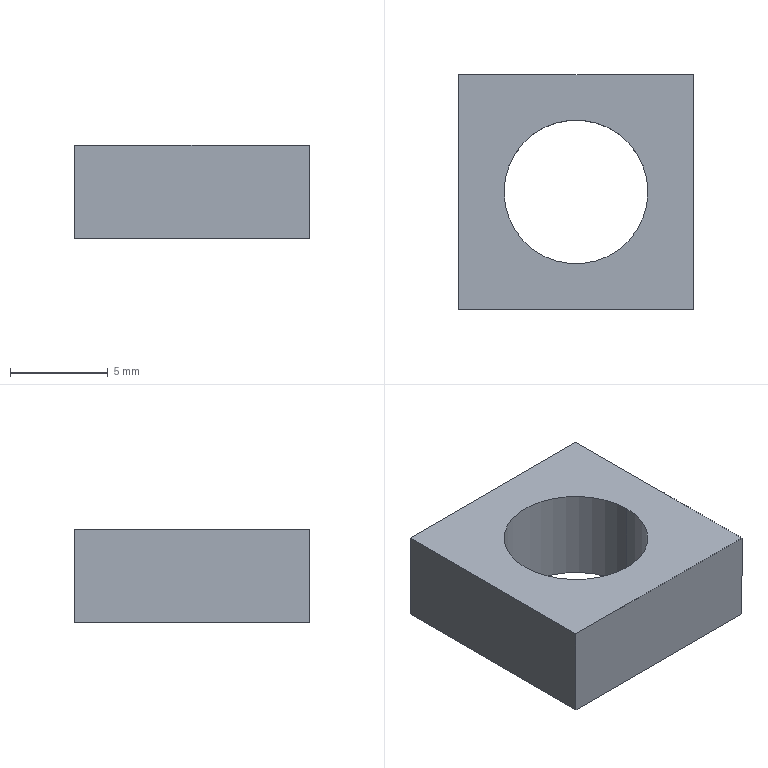Part | SolidWorks | features Extrusion 1 | 1 solid | 8 faces | box 12 x 12 x 4.756 mm | volume 483.113 mm3 | plane 6 | cylinder 2 | commonest cylinder face diameters 7.349 x2
STEP:
#1=CARTESIAN_POINT('',(15.877,1.837,4.756));
#2=VERTEX_POINT('',#1);
#3=CARTESIAN_POINT('',(23.226,1.837,4.756));
#4=VERTEX_POINT('',#3);
#5=CARTESIAN_POINT('',(19.552,1.837,4.756));
#6=DIRECTION('',(0.,0.,1.));
#7=DIRECTION('',(1.,0.,0.));
#8=AXIS2_PLACEMENT_3D('',#5,#6,#7);
#9=CIRCLE('',#8,3.675);
#10=EDGE_CURVE('',#2,#4,#9,.T.);
#11=ORIENTED_EDGE('',*,*,#10,.T.);
#12=CARTESIAN_POINT('',(23.226,1.837,0.));
#13=VERTEX_POINT('',#12);
#14=CARTESIAN_POINT('',(23.226,1.837,21.727));
#15=DIRECTION('',(0.,0.,-1.));
#16=VECTOR('',#15,1000.);
#17=LINE('',#14,#16);
#18=EDGE_CURVE('',#4,#13,#17,.T.);
#19=ORIENTED_EDGE('',*,*,#18,.T.);
#20=CARTESIAN_POINT('',(15.877,1.837,0.));
#21=VERTEX_POINT('',#20);
#22=CARTESIAN_POINT('',(19.552,1.837,0.));
#23=DIRECTION('',(0.,0.,1.));
#24=DIRECTION('',(1.,0.,0.));
#25=AXIS2_PLACEMENT_3D('',#22,#23,#24);
#26=CIRCLE('',#25,3.675);
#27=EDGE_CURVE('',#21,#13,#26,.T.);
#28=ORIENTED_EDGE('',*,*,#27,.F.);
#29=CARTESIAN_POINT('',(15.877,1.837,21.727));
#30=DIRECTION('',(0.,0.,-1.));
#31=VECTOR('',#30,1000.);
#32=LINE('',#29,#31);
#33=EDGE_CURVE('',#2,#21,#32,.T.);
#34=ORIENTED_EDGE('',*,*,#33,.F.);
#35=EDGE_LOOP('',(#11,#19,#28,#34));
#36=FACE_OUTER_BOUND('',#35,.T.);
#37=CARTESIAN_POINT('',(19.552,1.837,21.727));
#38=DIRECTION('',(0.,0.,-1.));
#39=DIRECTION('',(-1.,0.,0.));
#40=AXIS2_PLACEMENT_3D('',#37,#38,#39);
#41=CYLINDRICAL_SURFACE('',#40,3.675);
#42=ADVANCED_FACE('',(#36),#41,.F.);
#43=CARTESIAN_POINT('',(13.552,-4.163,4.756));
#44=VERTEX_POINT('',#43);
#45=CARTESIAN_POINT('',(25.552,-4.163,4.756));
#46=VERTEX_POINT('',#45);
#47=CARTESIAN_POINT('',(13.552,-4.163,4.756));
#48=DIRECTION('',(1.,0.,0.));
#49=VECTOR('',#48,1000.);
#50=LINE('',#47,#49);
#51=EDGE_CURVE('',#44,#46,#50,.T.);
#52=ORIENTED_EDGE('',*,*,#51,.F.);
#53=CARTESIAN_POINT('',(13.552,-4.163,0.));
#54=VERTEX_POINT('',#53);
#55=CARTESIAN_POINT('',(13.552,-4.163,21.727));
#56=DIRECTION('',(0.,0.,-1.));
#57=VECTOR('',#56,1000.);
#58=LINE('',#55,#57);
#59=EDGE_CURVE('',#44,#54,#58,.T.);
#60=ORIENTED_EDGE('',*,*,#59,.T.);
#61=CARTESIAN_POINT('',(25.552,-4.163,0.));
#62=VERTEX_POINT('',#61);
#63=CARTESIAN_POINT('',(13.552,-4.163,0.));
#64=DIRECTION('',(1.,0.,0.));
#65=VECTOR('',#64,1000.);
#66=LINE('',#63,#65);
#67=EDGE_CURVE('',#54,#62,#66,.T.);
#68=ORIENTED_EDGE('',*,*,#67,.T.);
#69=CARTESIAN_POINT('',(25.552,-4.163,21.727));
#70=DIRECTION('',(0.,0.,-1.));
#71=VECTOR('',#70,1000.);
#72=LINE('',#69,#71);
#73=EDGE_CURVE('',#46,#62,#72,.T.);
#74=ORIENTED_EDGE('',*,*,#73,.F.);
#75=EDGE_LOOP('',(#52,#60,#68,#74));
#76=FACE_OUTER_BOUND('',#75,.T.);
#77=CARTESIAN_POINT('',(13.552,-4.163,21.727));
#78=DIRECTION('',(0.,1.,0.));
#79=DIRECTION('',(0.,0.,1.));
#80=AXIS2_PLACEMENT_3D('',#77,#78,#79);
#81=PLANE('',#80);
#82=ADVANCED_FACE('',(#76),#81,.F.);
#83=CARTESIAN_POINT('',(13.552,7.837,4.756));
#84=VERTEX_POINT('',#83);
#85=CARTESIAN_POINT('',(13.552,7.837,4.756));
#86=DIRECTION('',(0.,-1.,0.));
#87=VECTOR('',#86,1000.);
#88=LINE('',#85,#87);
#89=EDGE_CURVE('',#84,#44,#88,.T.);
#90=ORIENTED_EDGE('',*,*,#89,.F.);
#91=CARTESIAN_POINT('',(13.552,7.837,0.));
#92=VERTEX_POINT('',#91);
#93=CARTESIAN_POINT('',(13.552,7.837,21.727));
#94=DIRECTION('',(0.,0.,-1.));
#95=VECTOR('',#94,1000.);
#96=LINE('',#93,#95);
#97=EDGE_CURVE('',#84,#92,#96,.T.);
#98=ORIENTED_EDGE('',*,*,#97,.T.);
#99=CARTESIAN_POINT('',(13.552,7.837,0.));
#100=DIRECTION('',(0.,-1.,0.));
#101=VECTOR('',#100,1000.);
#102=LINE('',#99,#101);
#103=EDGE_CURVE('',#92,#54,#102,.T.);
#104=ORIENTED_EDGE('',*,*,#103,.T.);
#105=ORIENTED_EDGE('',*,*,#59,.F.);
#106=EDGE_LOOP('',(#90,#98,#104,#105));
#107=FACE_OUTER_BOUND('',#106,.T.);
#108=CARTESIAN_POINT('',(13.552,7.837,21.727));
#109=DIRECTION('',(1.,0.,0.));
#110=DIRECTION('',(0.,0.,-1.));
#111=AXIS2_PLACEMENT_3D('',#108,#109,#110);
#112=PLANE('',#111);
#113=ADVANCED_FACE('',(#107),#112,.F.);
#114=CARTESIAN_POINT('',(25.552,7.837,4.756));
#115=VERTEX_POINT('',#114);
#116=CARTESIAN_POINT('',(25.552,7.837,4.756));
#117=DIRECTION('',(-1.,0.,0.));
#118=VECTOR('',#117,1000.);
#119=LINE('',#116,#118);
#120=EDGE_CURVE('',#115,#84,#119,.T.);
#121=ORIENTED_EDGE('',*,*,#120,.F.);
#122=CARTESIAN_POINT('',(25.552,7.837,0.));
#123=VERTEX_POINT('',#122);
#124=CARTESIAN_POINT('',(25.552,7.837,21.727));
#125=DIRECTION('',(0.,0.,-1.));
#126=VECTOR('',#125,1000.);
#127=LINE('',#124,#126);
#128=EDGE_CURVE('',#115,#123,#127,.T.);
#129=ORIENTED_EDGE('',*,*,#128,.T.);
#130=CARTESIAN_POINT('',(25.552,7.837,0.));
#131=DIRECTION('',(-1.,0.,0.));
#132=VECTOR('',#131,1000.);
#133=LINE('',#130,#132);
#134=EDGE_CURVE('',#123,#92,#133,.T.);
#135=ORIENTED_EDGE('',*,*,#134,.T.);
#136=ORIENTED_EDGE('',*,*,#97,.F.);
#137=EDGE_LOOP('',(#121,#129,#135,#136));
#138=FACE_OUTER_BOUND('',#137,.T.);
#139=CARTESIAN_POINT('',(25.552,7.837,21.727));
#140=DIRECTION('',(0.,-1.,0.));
#141=DIRECTION('',(0.,0.,-1.));
#142=AXIS2_PLACEMENT_3D('',#139,#140,#141);
#143=PLANE('',#142);
#144=ADVANCED_FACE('',(#138),#143,.F.);
#145=CARTESIAN_POINT('',(25.552,-4.163,4.756));
#146=DIRECTION('',(0.,1.,0.));
#147=VECTOR('',#146,1000.);
#148=LINE('',#145,#147);
#149=EDGE_CURVE('',#46,#115,#148,.T.);
#150=ORIENTED_EDGE('',*,*,#149,.F.);
#151=ORIENTED_EDGE('',*,*,#73,.T.);
#152=CARTESIAN_POINT('',(25.552,-4.163,0.));
#153=DIRECTION('',(0.,1.,0.));
#154=VECTOR('',#153,1000.);
#155=LINE('',#152,#154);
#156=EDGE_CURVE('',#62,#123,#155,.T.);
#157=ORIENTED_EDGE('',*,*,#156,.T.);
#158=ORIENTED_EDGE('',*,*,#128,.F.);
#159=EDGE_LOOP('',(#150,#151,#157,#158));
#160=FACE_OUTER_BOUND('',#159,.T.);
#161=CARTESIAN_POINT('',(25.552,-4.163,21.727));
#162=DIRECTION('',(-1.,0.,0.));
#163=DIRECTION('',(0.,-1.,0.));
#164=AXIS2_PLACEMENT_3D('',#161,#162,#163);
#165=PLANE('',#164);
#166=ADVANCED_FACE('',(#160),#165,.F.);
#167=ORIENTED_EDGE('',*,*,#156,.F.);
#168=ORIENTED_EDGE('',*,*,#67,.F.);
#169=ORIENTED_EDGE('',*,*,#103,.F.);
#170=ORIENTED_EDGE('',*,*,#134,.F.);
#171=EDGE_LOOP('',(#167,#168,#169,#170));
#172=FACE_OUTER_BOUND('',#171,.T.);
#173=ORIENTED_EDGE('',*,*,#27,.T.);
#174=CARTESIAN_POINT('',(19.552,1.837,0.));
#175=DIRECTION('',(0.,0.,1.));
#176=DIRECTION('',(1.,0.,0.));
#177=AXIS2_PLACEMENT_3D('',#174,#175,#176);
#178=CIRCLE('',#177,3.675);
#179=EDGE_CURVE('',#13,#21,#178,.T.);
#180=ORIENTED_EDGE('',*,*,#179,.T.);
#181=EDGE_LOOP('',(#173,#180));
#182=FACE_BOUND('',#181,.T.);
#183=CARTESIAN_POINT('',(0.,0.,0.));
#184=DIRECTION('',(0.,0.,1.));
#185=DIRECTION('',(1.,0.,0.));
#186=AXIS2_PLACEMENT_3D('',#183,#184,#185);
#187=PLANE('',#186);
#188=ADVANCED_FACE('',(#172,#182),#187,.F.);
#189=ORIENTED_EDGE('',*,*,#18,.F.);
#190=CARTESIAN_POINT('',(19.552,1.837,4.756));
#191=DIRECTION('',(0.,0.,1.));
#192=DIRECTION('',(1.,0.,0.));
#193=AXIS2_PLACEMENT_3D('',#190,#191,#192);
#194=CIRCLE('',#193,3.675);
#195=EDGE_CURVE('',#4,#2,#194,.T.);
#196=ORIENTED_EDGE('',*,*,#195,.T.);
#197=ORIENTED_EDGE('',*,*,#33,.T.);
#198=ORIENTED_EDGE('',*,*,#179,.F.);
#199=EDGE_LOOP('',(#189,#196,#197,#198));
#200=FACE_OUTER_BOUND('',#199,.T.);
#201=CARTESIAN_POINT('',(19.552,1.837,21.727));
#202=DIRECTION('',(0.,0.,-1.));
#203=DIRECTION('',(-1.,0.,0.));
#204=AXIS2_PLACEMENT_3D('',#201,#202,#203);
#205=CYLINDRICAL_SURFACE('',#204,3.675);
#206=ADVANCED_FACE('',(#200),#205,.F.);
#207=ORIENTED_EDGE('',*,*,#10,.F.);
#208=ORIENTED_EDGE('',*,*,#195,.F.);
#209=EDGE_LOOP('',(#207,#208));
#210=FACE_BOUND('',#209,.T.);
#211=ORIENTED_EDGE('',*,*,#51,.T.);
#212=ORIENTED_EDGE('',*,*,#149,.T.);
#213=ORIENTED_EDGE('',*,*,#120,.T.);
#214=ORIENTED_EDGE('',*,*,#89,.T.);
#215=EDGE_LOOP('',(#211,#212,#213,#214));
#216=FACE_OUTER_BOUND('',#215,.T.);
#217=CARTESIAN_POINT('',(19.552,1.837,4.756));
#218=DIRECTION('',(0.,0.,1.));
#219=DIRECTION('',(-0.4657,-0.8849,0.));
#220=AXIS2_PLACEMENT_3D('',#217,#218,#219);
#221=PLANE('',#220);
#222=ADVANCED_FACE('',(#210,#216),#221,.T.);
#223=CLOSED_SHELL('',(#42,#82,#113,#144,#166,#188,#206,#222));
#224=MANIFOLD_SOLID_BREP('',#223);
#225=CARTESIAN_POINT('',(0.,0.,0.));
#226=DIRECTION('',(0.,0.,1.));
#227=DIRECTION('',(1.,0.,0.));
#228=AXIS2_PLACEMENT_3D('',#225,#226,#227);
#229=(LENGTH_UNIT()NAMED_UNIT(*)SI_UNIT(.MILLI.,.METRE.));
#230=UNCERTAINTY_MEASURE_WITH_UNIT(LENGTH_MEASURE(0.00001),#229,'','');
#231=(NAMED_UNIT(*)PLANE_ANGLE_UNIT()SI_UNIT($,.RADIAN.));
#232=(NAMED_UNIT(*)SI_UNIT($,.STERADIAN.)SOLID_ANGLE_UNIT());
#233=(GEOMETRIC_REPRESENTATION_CONTEXT(3)GLOBAL_UNCERTAINTY_ASSIGNED_CONTEXT((#230))GLOBAL_UNIT_ASSIGNED_CONTEXT((#229,#231,#232))REPRESENTATION_CONTEXT('',''));
#234=ADVANCED_BREP_SHAPE_REPRESENTATION('',(#224,#228),#233);